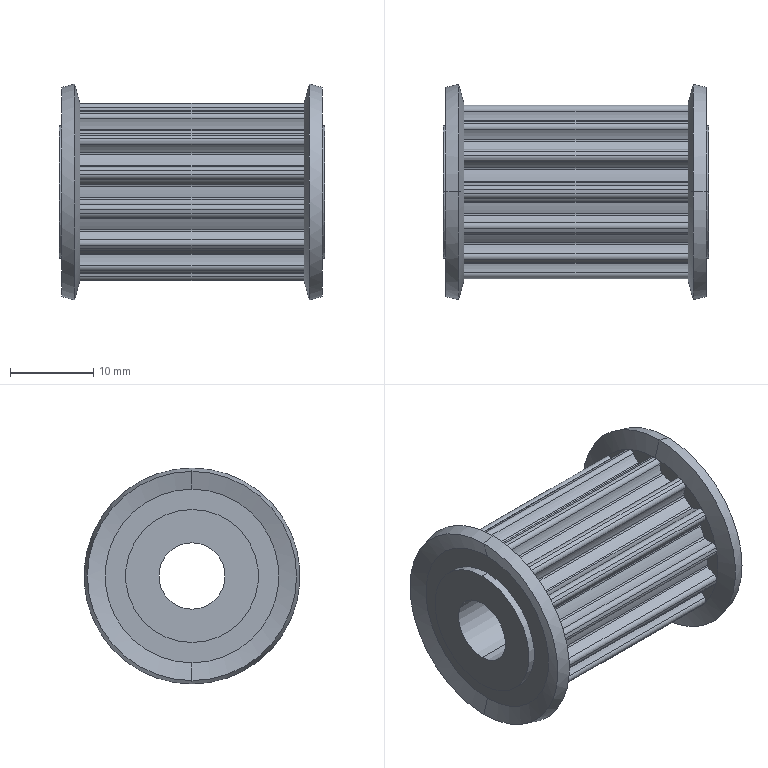Part | SolidWorks | 1 solid | 163 faces | box 32 x 26 x 26 mm | volume 8249 mm3 | cylinder 119 | plane 32 | cone 12 | commonest cylinder face diameters 0.5 x28 1.1 x28 6.55 x28 21.32 x15 17.78 x14 16 x4